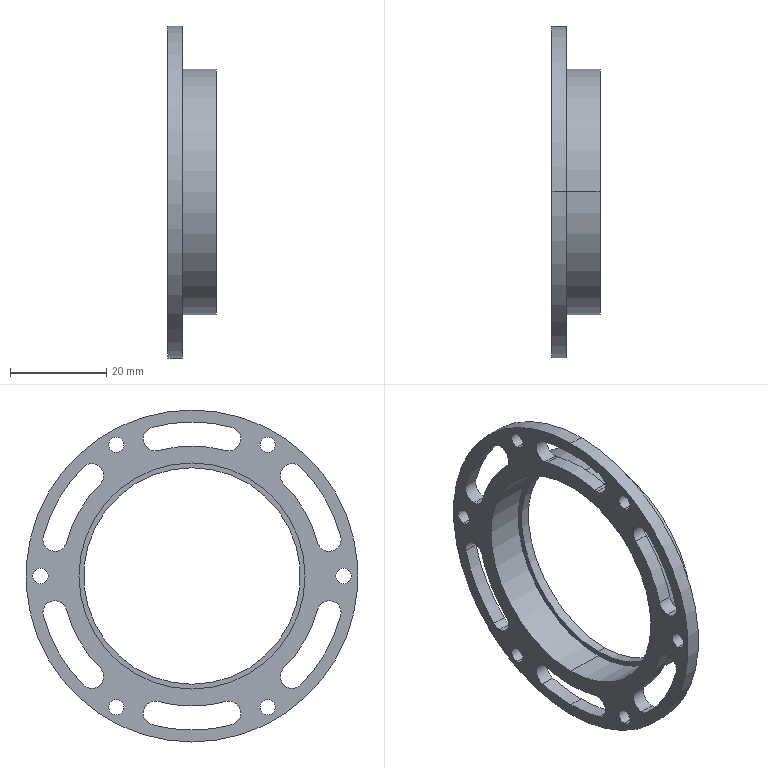Part | SolidWorks | features ICE 2, Revolution 1 | 1 solid | 56 faces | box 10 x 69 x 69 mm | volume 6569 mm3 | cylinder 52 | plane 4 | commonest cylinder face diameters 5 x18 3.2 x12 54 x7 64 x7 45 x2 47 x2